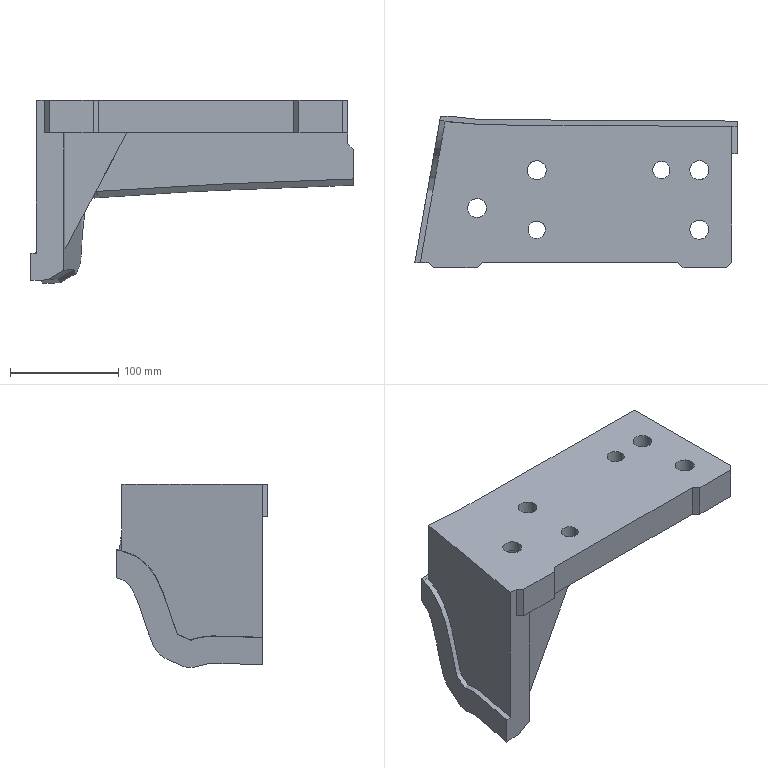Part | NX | features solid 2 | 1 solid | 44 faces | box 297.454 x 139.786 x 169.006 mm | volume 1831039 mm3 | plane 23 | cylinder 11 | spline 10 | commonest cylinder face diameters 17.5 x4 25 x4 16 x2 30 x1